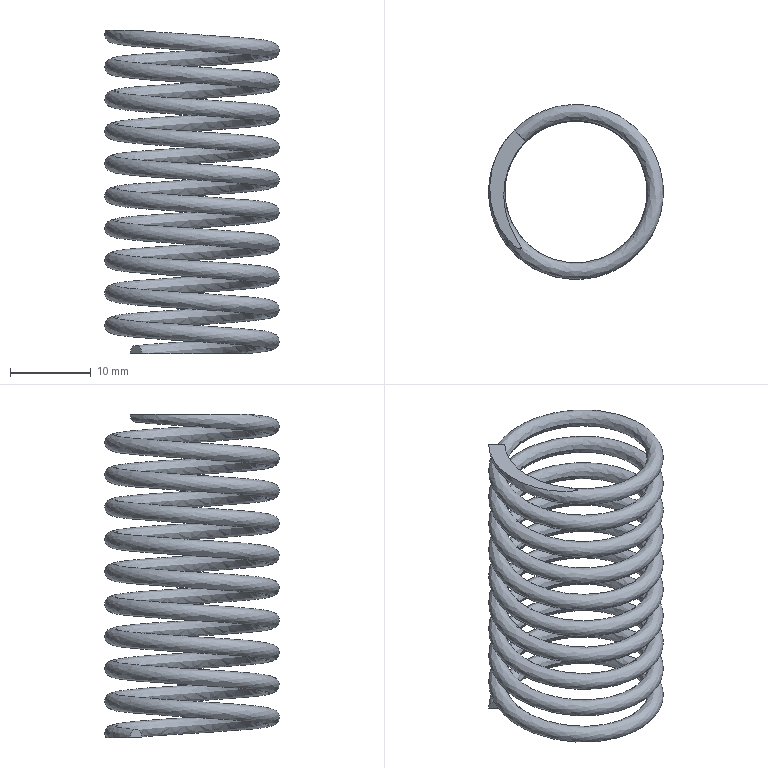Part | STEP file | tieqiantanhuang | 1 solid | 5 faces | box 21.623 x 21.623 x 40 mm | volume 1892 mm3 | plane 4 | spline 1